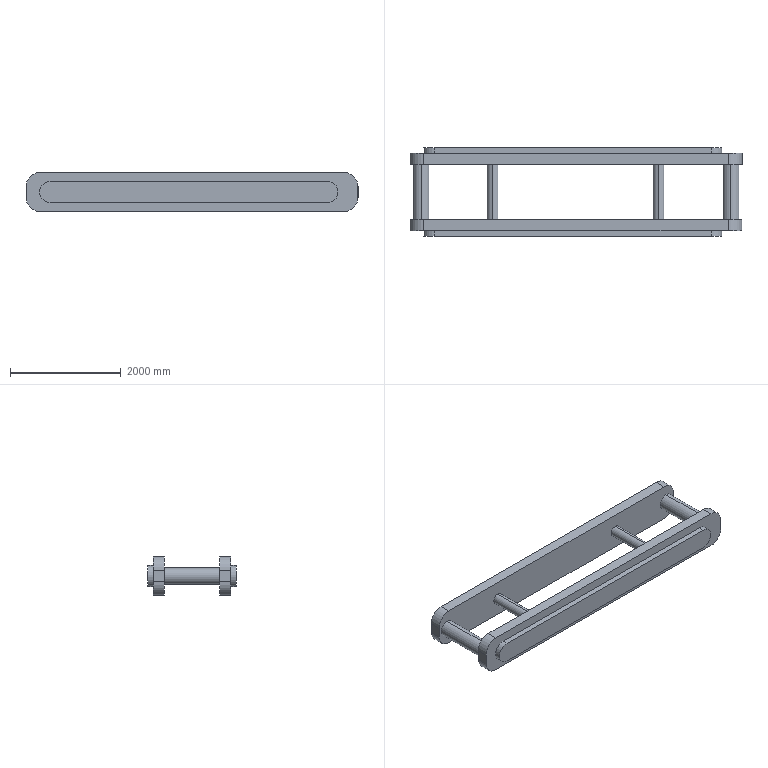Part | SolidWorks | features ICE 3, Extrusion 1, Fillet 1, MirrorPattern 1 | 1 solid | 38 faces | box 6002 x 1600 x 700 mm | volume 2271942121 mm3 | cylinder 20 | plane 18 | commonest cylinder face diameters 500 x8 200 x4 300 x4 384.606 x4
STEP:
#1=CARTESIAN_POINT('',(-2800.,1200.,150.));
#2=VERTEX_POINT('',#1);
#3=CARTESIAN_POINT('',(-2800.,1200.,-150.));
#4=VERTEX_POINT('',#3);
#5=CARTESIAN_POINT('',(-2800.,1200.,0.));
#6=DIRECTION('',(0.,1.,0.));
#7=DIRECTION('',(0.,0.,1.));
#8=AXIS2_PLACEMENT_3D('',#5,#6,#7);
#9=CIRCLE('',#8,150.);
#10=EDGE_CURVE('',#2,#4,#9,.T.);
#11=ORIENTED_EDGE('',*,*,#10,.F.);
#12=CARTESIAN_POINT('',(-2800.,200.,150.));
#13=VERTEX_POINT('',#12);
#14=CARTESIAN_POINT('',(-2800.,1200.,150.));
#15=DIRECTION('',(0.,-1.,0.));
#16=VECTOR('',#15,1000.);
#17=LINE('',#14,#16);
#18=EDGE_CURVE('',#2,#13,#17,.T.);
#19=ORIENTED_EDGE('',*,*,#18,.T.);
#20=CARTESIAN_POINT('',(-2800.,200.,-150.));
#21=VERTEX_POINT('',#20);
#22=CARTESIAN_POINT('',(-2800.,200.,0.));
#23=DIRECTION('',(0.,1.,0.));
#24=DIRECTION('',(0.,0.,1.));
#25=AXIS2_PLACEMENT_3D('',#22,#23,#24);
#26=CIRCLE('',#25,150.);
#27=EDGE_CURVE('',#13,#21,#26,.T.);
#28=ORIENTED_EDGE('',*,*,#27,.T.);
#29=CARTESIAN_POINT('',(-2800.,1200.,-150.));
#30=DIRECTION('',(0.,-1.,0.));
#31=VECTOR('',#30,1000.);
#32=LINE('',#29,#31);
#33=EDGE_CURVE('',#4,#21,#32,.T.);
#34=ORIENTED_EDGE('',*,*,#33,.F.);
#35=EDGE_LOOP('',(#11,#19,#28,#34));
#36=FACE_OUTER_BOUND('',#35,.T.);
#37=CARTESIAN_POINT('',(-2800.,1200.,0.));
#38=DIRECTION('',(0.,-1.,0.));
#39=DIRECTION('',(0.,0.,-1.));
#40=AXIS2_PLACEMENT_3D('',#37,#38,#39);
#41=CYLINDRICAL_SURFACE('',#40,150.);
#42=ADVANCED_FACE('',(#36),#41,.T.);
#43=CARTESIAN_POINT('',(1500.,1200.,100.));
#44=VERTEX_POINT('',#43);
#45=CARTESIAN_POINT('',(1500.,1200.,-100.));
#46=VERTEX_POINT('',#45);
#47=CARTESIAN_POINT('',(1500.,1200.,0.));
#48=DIRECTION('',(0.,1.,0.));
#49=DIRECTION('',(0.,0.,1.));
#50=AXIS2_PLACEMENT_3D('',#47,#48,#49);
#51=CIRCLE('',#50,100.);
#52=EDGE_CURVE('',#44,#46,#51,.T.);
#53=ORIENTED_EDGE('',*,*,#52,.F.);
#54=CARTESIAN_POINT('',(1500.,200.,100.));
#55=VERTEX_POINT('',#54);
#56=CARTESIAN_POINT('',(1500.,1200.,100.));
#57=DIRECTION('',(0.,-1.,0.));
#58=VECTOR('',#57,1000.);
#59=LINE('',#56,#58);
#60=EDGE_CURVE('',#44,#55,#59,.T.);
#61=ORIENTED_EDGE('',*,*,#60,.T.);
#62=CARTESIAN_POINT('',(1500.,200.,-100.));
#63=VERTEX_POINT('',#62);
#64=CARTESIAN_POINT('',(1500.,200.,0.));
#65=DIRECTION('',(0.,1.,0.));
#66=DIRECTION('',(0.,0.,1.));
#67=AXIS2_PLACEMENT_3D('',#64,#65,#66);
#68=CIRCLE('',#67,100.);
#69=EDGE_CURVE('',#55,#63,#68,.T.);
#70=ORIENTED_EDGE('',*,*,#69,.T.);
#71=CARTESIAN_POINT('',(1500.,1200.,-100.));
#72=DIRECTION('',(0.,-1.,0.));
#73=VECTOR('',#72,1000.);
#74=LINE('',#71,#73);
#75=EDGE_CURVE('',#46,#63,#74,.T.);
#76=ORIENTED_EDGE('',*,*,#75,.F.);
#77=EDGE_LOOP('',(#53,#61,#70,#76));
#78=FACE_OUTER_BOUND('',#77,.T.);
#79=CARTESIAN_POINT('',(1500.,1200.,0.));
#80=DIRECTION('',(0.,-1.,0.));
#81=DIRECTION('',(0.,0.,-1.));
#82=AXIS2_PLACEMENT_3D('',#79,#80,#81);
#83=CYLINDRICAL_SURFACE('',#82,100.);
#84=ADVANCED_FACE('',(#78),#83,.T.);
#85=CARTESIAN_POINT('',(-1500.,1200.,100.));
#86=VERTEX_POINT('',#85);
#87=CARTESIAN_POINT('',(-1500.,1200.,-100.));
#88=VERTEX_POINT('',#87);
#89=CARTESIAN_POINT('',(-1500.,1200.,0.));
#90=DIRECTION('',(0.,1.,0.));
#91=DIRECTION('',(0.,0.,1.));
#92=AXIS2_PLACEMENT_3D('',#89,#90,#91);
#93=CIRCLE('',#92,100.);
#94=EDGE_CURVE('',#86,#88,#93,.T.);
#95=ORIENTED_EDGE('',*,*,#94,.F.);
#96=CARTESIAN_POINT('',(-1500.,200.,100.));
#97=VERTEX_POINT('',#96);
#98=CARTESIAN_POINT('',(-1500.,1200.,100.));
#99=DIRECTION('',(0.,-1.,0.));
#100=VECTOR('',#99,1000.);
#101=LINE('',#98,#100);
#102=EDGE_CURVE('',#86,#97,#101,.T.);
#103=ORIENTED_EDGE('',*,*,#102,.T.);
#104=CARTESIAN_POINT('',(-1500.,200.,-100.));
#105=VERTEX_POINT('',#104);
#106=CARTESIAN_POINT('',(-1500.,200.,0.));
#107=DIRECTION('',(0.,1.,0.));
#108=DIRECTION('',(0.,0.,1.));
#109=AXIS2_PLACEMENT_3D('',#106,#107,#108);
#110=CIRCLE('',#109,100.);
#111=EDGE_CURVE('',#97,#105,#110,.T.);
#112=ORIENTED_EDGE('',*,*,#111,.T.);
#113=CARTESIAN_POINT('',(-1500.,1200.,-100.));
#114=DIRECTION('',(0.,-1.,0.));
#115=VECTOR('',#114,1000.);
#116=LINE('',#113,#115);
#117=EDGE_CURVE('',#88,#105,#116,.T.);
#118=ORIENTED_EDGE('',*,*,#117,.F.);
#119=EDGE_LOOP('',(#95,#103,#112,#118));
#120=FACE_OUTER_BOUND('',#119,.T.);
#121=CARTESIAN_POINT('',(-1500.,1200.,0.));
#122=DIRECTION('',(0.,-1.,0.));
#123=DIRECTION('',(0.,0.,-1.));
#124=AXIS2_PLACEMENT_3D('',#121,#122,#123);
#125=CYLINDRICAL_SURFACE('',#124,100.);
#126=ADVANCED_FACE('',(#120),#125,.T.);
#127=CARTESIAN_POINT('',(2800.,1200.,150.));
#128=VERTEX_POINT('',#127);
#129=CARTESIAN_POINT('',(2800.,1200.,-150.));
#130=VERTEX_POINT('',#129);
#131=CARTESIAN_POINT('',(2800.,1200.,0.));
#132=DIRECTION('',(0.,1.,0.));
#133=DIRECTION('',(0.,0.,1.));
#134=AXIS2_PLACEMENT_3D('',#131,#132,#133);
#135=CIRCLE('',#134,150.);
#136=EDGE_CURVE('',#128,#130,#135,.T.);
#137=ORIENTED_EDGE('',*,*,#136,.F.);
#138=CARTESIAN_POINT('',(2800.,200.,150.));
#139=VERTEX_POINT('',#138);
#140=CARTESIAN_POINT('',(2800.,1200.,150.));
#141=DIRECTION('',(0.,-1.,0.));
#142=VECTOR('',#141,1000.);
#143=LINE('',#140,#142);
#144=EDGE_CURVE('',#128,#139,#143,.T.);
#145=ORIENTED_EDGE('',*,*,#144,.T.);
#146=CARTESIAN_POINT('',(2800.,200.,-150.));
#147=VERTEX_POINT('',#146);
#148=CARTESIAN_POINT('',(2800.,200.,0.));
#149=DIRECTION('',(0.,1.,0.));
#150=DIRECTION('',(0.,0.,1.));
#151=AXIS2_PLACEMENT_3D('',#148,#149,#150);
#152=CIRCLE('',#151,150.);
#153=EDGE_CURVE('',#139,#147,#152,.T.);
#154=ORIENTED_EDGE('',*,*,#153,.T.);
#155=CARTESIAN_POINT('',(2800.,1200.,-150.));
#156=DIRECTION('',(0.,-1.,0.));
#157=VECTOR('',#156,1000.);
#158=LINE('',#155,#157);
#159=EDGE_CURVE('',#130,#147,#158,.T.);
#160=ORIENTED_EDGE('',*,*,#159,.F.);
#161=EDGE_LOOP('',(#137,#145,#154,#160));
#162=FACE_OUTER_BOUND('',#161,.T.);
#163=CARTESIAN_POINT('',(2800.,1200.,0.));
#164=DIRECTION('',(0.,-1.,0.));
#165=DIRECTION('',(0.,0.,-1.));
#166=AXIS2_PLACEMENT_3D('',#163,#164,#165);
#167=CYLINDRICAL_SURFACE('',#166,150.);
#168=ADVANCED_FACE('',(#162),#167,.T.);
#169=CARTESIAN_POINT('',(2750.,0.,-350.));
#170=VERTEX_POINT('',#169);
#171=CARTESIAN_POINT('',(-2750.,0.,-350.));
#172=VERTEX_POINT('',#171);
#173=CARTESIAN_POINT('',(-3000.,0.,-350.));
#174=DIRECTION('',(-1.,0.,0.));
#175=VECTOR('',#174,1000.);
#176=LINE('',#173,#175);
#177=EDGE_CURVE('',#170,#172,#176,.T.);
#178=ORIENTED_EDGE('',*,*,#177,.F.);
#179=CARTESIAN_POINT('',(3000.,0.,-100.));
#180=VERTEX_POINT('',#179);
#181=CARTESIAN_POINT('',(2750.,0.,-100.));
#182=DIRECTION('',(0.,-1.,0.));
#183=DIRECTION('',(0.,0.,1.));
#184=AXIS2_PLACEMENT_3D('',#181,#182,#183);
#185=CIRCLE('',#184,250.);
#186=EDGE_CURVE('',#170,#180,#185,.T.);
#187=ORIENTED_EDGE('',*,*,#186,.T.);
#188=CARTESIAN_POINT('',(3000.,0.,100.));
#189=VERTEX_POINT('',#188);
#190=CARTESIAN_POINT('',(3000.,0.,-350.));
#191=DIRECTION('',(0.,0.,-1.));
#192=VECTOR('',#191,1000.);
#193=LINE('',#190,#192);
#194=EDGE_CURVE('',#189,#180,#193,.T.);
#195=ORIENTED_EDGE('',*,*,#194,.F.);
#196=CARTESIAN_POINT('',(2750.,0.,350.));
#197=VERTEX_POINT('',#196);
#198=CARTESIAN_POINT('',(2750.,0.,100.));
#199=DIRECTION('',(0.,-1.,0.));
#200=DIRECTION('',(0.,0.,1.));
#201=AXIS2_PLACEMENT_3D('',#198,#199,#200);
#202=CIRCLE('',#201,250.);
#203=EDGE_CURVE('',#189,#197,#202,.T.);
#204=ORIENTED_EDGE('',*,*,#203,.T.);
#205=CARTESIAN_POINT('',(-2750.,0.,350.));
#206=VERTEX_POINT('',#205);
#207=CARTESIAN_POINT('',(-3000.,0.,350.));
#208=DIRECTION('',(1.,0.,0.));
#209=VECTOR('',#208,1000.);
#210=LINE('',#207,#209);
#211=EDGE_CURVE('',#206,#197,#210,.T.);
#212=ORIENTED_EDGE('',*,*,#211,.F.);
#213=CARTESIAN_POINT('',(-3000.,0.,100.));
#214=VERTEX_POINT('',#213);
#215=CARTESIAN_POINT('',(-2750.,0.,100.));
#216=DIRECTION('',(0.,-1.,0.));
#217=DIRECTION('',(0.,0.,1.));
#218=AXIS2_PLACEMENT_3D('',#215,#216,#217);
#219=CIRCLE('',#218,250.);
#220=EDGE_CURVE('',#206,#214,#219,.T.);
#221=ORIENTED_EDGE('',*,*,#220,.T.);
#222=CARTESIAN_POINT('',(-3000.,0.,-100.));
#223=VERTEX_POINT('',#222);
#224=CARTESIAN_POINT('',(-3000.,0.,-350.));
#225=DIRECTION('',(0.,0.,1.));
#226=VECTOR('',#225,1000.);
#227=LINE('',#224,#226);
#228=EDGE_CURVE('',#223,#214,#227,.T.);
#229=ORIENTED_EDGE('',*,*,#228,.F.);
#230=CARTESIAN_POINT('',(-2750.,0.,-100.));
#231=DIRECTION('',(0.,-1.,0.));
#232=DIRECTION('',(0.,0.,1.));
#233=AXIS2_PLACEMENT_3D('',#230,#231,#232);
#234=CIRCLE('',#233,250.);
#235=EDGE_CURVE('',#223,#172,#234,.T.);
#236=ORIENTED_EDGE('',*,*,#235,.T.);
#237=EDGE_LOOP('',(#178,#187,#195,#204,#212,#221,#229,#236));
#238=FACE_OUTER_BOUND('',#237,.T.);
#239=CARTESIAN_POINT('',(-2564.073,0.,192.303));
#240=VERTEX_POINT('',#239);
#241=CARTESIAN_POINT('',(-2564.073,0.,-192.303));
#242=VERTEX_POINT('',#241);
#243=CARTESIAN_POINT('',(-2564.073,0.,0.));
#244=DIRECTION('',(0.,-1.,0.));
#245=DIRECTION('',(0.,0.,-1.));
#246=AXIS2_PLACEMENT_3D('',#243,#244,#245);
#247=CIRCLE('',#246,192.303);
#248=EDGE_CURVE('',#240,#242,#247,.T.);
#249=ORIENTED_EDGE('',*,*,#248,.F.);
#250=CARTESIAN_POINT('',(2449.537,0.,192.303));
#251=VERTEX_POINT('',#250);
#252=CARTESIAN_POINT('',(-2564.073,0.,192.303));
#253=DIRECTION('',(-1.,0.,0.));
#254=VECTOR('',#253,1000.);
#255=LINE('',#252,#254);
#256=EDGE_CURVE('',#251,#240,#255,.T.);
#257=ORIENTED_EDGE('',*,*,#256,.F.);
#258=CARTESIAN_POINT('',(2449.537,0.,-192.303));
#259=VERTEX_POINT('',#258);
#260=CARTESIAN_POINT('',(2449.537,0.,0.));
#261=DIRECTION('',(0.,-1.,0.));
#262=DIRECTION('',(0.,0.,-1.));
#263=AXIS2_PLACEMENT_3D('',#260,#261,#262);
#264=CIRCLE('',#263,192.303);
#265=EDGE_CURVE('',#259,#251,#264,.T.);
#266=ORIENTED_EDGE('',*,*,#265,.F.);
#267=CARTESIAN_POINT('',(-2564.073,0.,-192.303));
#268=DIRECTION('',(1.,0.,0.));
#269=VECTOR('',#268,1000.);
#270=LINE('',#267,#269);
#271=EDGE_CURVE('',#242,#259,#270,.T.);
#272=ORIENTED_EDGE('',*,*,#271,.F.);
#273=EDGE_LOOP('',(#249,#257,#266,#272));
#274=FACE_BOUND('',#273,.T.);
#275=CARTESIAN_POINT('',(0.,0.,0.));
#276=DIRECTION('',(0.,1.,0.));
#277=DIRECTION('',(0.,0.,1.));
#278=AXIS2_PLACEMENT_3D('',#275,#276,#277);
#279=PLANE('',#278);
#280=ADVANCED_FACE('',(#238,#274),#279,.F.);
#281=ORIENTED_EDGE('',*,*,#194,.T.);
#282=CARTESIAN_POINT('',(3000.,200.,-100.));
#283=VERTEX_POINT('',#282);
#284=CARTESIAN_POINT('',(3000.,200.,-100.));
#285=DIRECTION('',(0.,1.,0.));
#286=VECTOR('',#285,1000.);
#287=LINE('',#284,#286);
#288=EDGE_CURVE('',#180,#283,#287,.T.);
#289=ORIENTED_EDGE('',*,*,#288,.T.);
#290=CARTESIAN_POINT('',(3000.,200.,100.));
#291=VERTEX_POINT('',#290);
#292=CARTESIAN_POINT('',(3000.,200.,-350.));
#293=DIRECTION('',(0.,0.,-1.));
#294=VECTOR('',#293,1000.);
#295=LINE('',#292,#294);
#296=EDGE_CURVE('',#291,#283,#295,.T.);
#297=ORIENTED_EDGE('',*,*,#296,.F.);
#298=CARTESIAN_POINT('',(3000.,200.,100.));
#299=DIRECTION('',(0.,-1.,0.));
#300=VECTOR('',#299,1000.);
#301=LINE('',#298,#300);
#302=EDGE_CURVE('',#291,#189,#301,.T.);
#303=ORIENTED_EDGE('',*,*,#302,.T.);
#304=EDGE_LOOP('',(#281,#289,#297,#303));
#305=FACE_OUTER_BOUND('',#304,.T.);
#306=CARTESIAN_POINT('',(3000.,200.,-350.));
#307=DIRECTION('',(-1.,0.,0.));
#308=DIRECTION('',(0.,0.,1.));
#309=AXIS2_PLACEMENT_3D('',#306,#307,#308);
#310=PLANE('',#309);
#311=ADVANCED_FACE('',(#305),#310,.F.);
#312=CARTESIAN_POINT('',(2750.,200.,-350.));
#313=VERTEX_POINT('',#312);
#314=CARTESIAN_POINT('',(-2750.,200.,-350.));
#315=VERTEX_POINT('',#314);
#316=CARTESIAN_POINT('',(-3000.,200.,-350.));
#317=DIRECTION('',(-1.,0.,0.));
#318=VECTOR('',#317,1000.);
#319=LINE('',#316,#318);
#320=EDGE_CURVE('',#313,#315,#319,.T.);
#321=ORIENTED_EDGE('',*,*,#320,.F.);
#322=CARTESIAN_POINT('',(2750.,200.,-350.));
#323=DIRECTION('',(0.,-1.,0.));
#324=VECTOR('',#323,1000.);
#325=LINE('',#322,#324);
#326=EDGE_CURVE('',#313,#170,#325,.T.);
#327=ORIENTED_EDGE('',*,*,#326,.T.);
#328=ORIENTED_EDGE('',*,*,#177,.T.);
#329=CARTESIAN_POINT('',(-2750.,200.,-350.));
#330=DIRECTION('',(0.,1.,0.));
#331=VECTOR('',#330,1000.);
#332=LINE('',#329,#331);
#333=EDGE_CURVE('',#172,#315,#332,.T.);
#334=ORIENTED_EDGE('',*,*,#333,.T.);
#335=EDGE_LOOP('',(#321,#327,#328,#334));
#336=FACE_OUTER_BOUND('',#335,.T.);
#337=CARTESIAN_POINT('',(-3000.,200.,-350.));
#338=DIRECTION('',(0.,0.,1.));
#339=DIRECTION('',(1.,0.,0.));
#340=AXIS2_PLACEMENT_3D('',#337,#338,#339);
#341=PLANE('',#340);
#342=ADVANCED_FACE('',(#336),#341,.F.);
#343=CARTESIAN_POINT('',(-3000.,200.,-100.));
#344=VERTEX_POINT('',#343);
#345=CARTESIAN_POINT('',(-3000.,200.,100.));
#346=VERTEX_POINT('',#345);
#347=CARTESIAN_POINT('',(-3000.,200.,-350.));
#348=DIRECTION('',(0.,0.,1.));
#349=VECTOR('',#348,1000.);
#350=LINE('',#347,#349);
#351=EDGE_CURVE('',#344,#346,#350,.T.);
#352=ORIENTED_EDGE('',*,*,#351,.F.);
#353=CARTESIAN_POINT('',(-3000.,200.,-100.));
#354=DIRECTION('',(0.,-1.,0.));
#355=VECTOR('',#354,1000.);
#356=LINE('',#353,#355);
#357=EDGE_CURVE('',#344,#223,#356,.T.);
#358=ORIENTED_EDGE('',*,*,#357,.T.);
#359=ORIENTED_EDGE('',*,*,#228,.T.);
#360=CARTESIAN_POINT('',(-3000.,200.,100.));
#361=DIRECTION('',(0.,1.,0.));
#362=VECTOR('',#361,1000.);
#363=LINE('',#360,#362);
#364=EDGE_CURVE('',#214,#346,#363,.T.);
#365=ORIENTED_EDGE('',*,*,#364,.T.);
#366=EDGE_LOOP('',(#352,#358,#359,#365));
#367=FACE_OUTER_BOUND('',#366,.T.);
#368=CARTESIAN_POINT('',(-3000.,200.,-350.));
#369=DIRECTION('',(1.,0.,0.));
#370=DIRECTION('',(0.,0.,-1.));
#371=AXIS2_PLACEMENT_3D('',#368,#369,#370);
#372=PLANE('',#371);
#373=ADVANCED_FACE('',(#367),#372,.F.);
#374=ORIENTED_EDGE('',*,*,#211,.T.);
#375=CARTESIAN_POINT('',(2750.,200.,350.));
#376=VERTEX_POINT('',#375);
#377=CARTESIAN_POINT('',(2750.,200.,350.));
#378=DIRECTION('',(0.,1.,0.));
#379=VECTOR('',#378,1000.);
#380=LINE('',#377,#379);
#381=EDGE_CURVE('',#197,#376,#380,.T.);
#382=ORIENTED_EDGE('',*,*,#381,.T.);
#383=CARTESIAN_POINT('',(-2750.,200.,350.));
#384=VERTEX_POINT('',#383);
#385=CARTESIAN_POINT('',(-3000.,200.,350.));
#386=DIRECTION('',(1.,0.,0.));
#387=VECTOR('',#386,1000.);
#388=LINE('',#385,#387);
#389=EDGE_CURVE('',#384,#376,#388,.T.);
#390=ORIENTED_EDGE('',*,*,#389,.F.);
#391=CARTESIAN_POINT('',(-2750.,200.,350.));
#392=DIRECTION('',(0.,-1.,0.));
#393=VECTOR('',#392,1000.);
#394=LINE('',#391,#393);
#395=EDGE_CURVE('',#384,#206,#394,.T.);
#396=ORIENTED_EDGE('',*,*,#395,.T.);
#397=EDGE_LOOP('',(#374,#382,#390,#396));
#398=FACE_OUTER_BOUND('',#397,.T.);
#399=CARTESIAN_POINT('',(-3000.,200.,350.));
#400=DIRECTION('',(0.,0.,-1.));
#401=DIRECTION('',(-1.,0.,0.));
#402=AXIS2_PLACEMENT_3D('',#399,#400,#401);
#403=PLANE('',#402);
#404=ADVANCED_FACE('',(#398),#403,.F.);
#405=CARTESIAN_POINT('',(-2800.,200.,0.));
#406=DIRECTION('',(0.,1.,0.));
#407=DIRECTION('',(0.,0.,1.));
#408=AXIS2_PLACEMENT_3D('',#405,#406,#407);
#409=CIRCLE('',#408,150.);
#410=EDGE_CURVE('',#21,#13,#409,.T.);
#411=ORIENTED_EDGE('',*,*,#410,.F.);
#412=ORIENTED_EDGE('',*,*,#27,.F.);
#413=EDGE_LOOP('',(#411,#412));
#414=FACE_BOUND('',#413,.T.);
#415=CARTESIAN_POINT('',(1500.,200.,0.));
#416=DIRECTION('',(0.,1.,0.));
#417=DIRECTION('',(0.,0.,1.));
#418=AXIS2_PLACEMENT_3D('',#415,#416,#417);
#419=CIRCLE('',#418,100.);
#420=EDGE_CURVE('',#63,#55,#419,.T.);
#421=ORIENTED_EDGE('',*,*,#420,.F.);
#422=ORIENTED_EDGE('',*,*,#69,.F.);
#423=EDGE_LOOP('',(#421,#422));
#424=FACE_BOUND('',#423,.T.);
#425=CARTESIAN_POINT('',(-1500.,200.,0.));
#426=DIRECTION('',(0.,1.,0.));
#427=DIRECTION('',(0.,0.,1.));
#428=AXIS2_PLACEMENT_3D('',#425,#426,#427);
#429=CIRCLE('',#428,100.);
#430=EDGE_CURVE('',#105,#97,#429,.T.);
#431=ORIENTED_EDGE('',*,*,#430,.F.);
#432=ORIENTED_EDGE('',*,*,#111,.F.);
#433=EDGE_LOOP('',(#431,#432));
#434=FACE_BOUND('',#433,.T.);
#435=CARTESIAN_POINT('',(2800.,200.,0.));
#436=DIRECTION('',(0.,1.,0.));
#437=DIRECTION('',(0.,0.,1.));
#438=AXIS2_PLACEMENT_3D('',#435,#436,#437);
#439=CIRCLE('',#438,150.);
#440=EDGE_CURVE('',#147,#139,#439,.T.);
#441=ORIENTED_EDGE('',*,*,#440,.F.);
#442=ORIENTED_EDGE('',*,*,#153,.F.);
#443=EDGE_LOOP('',(#441,#442));
#444=FACE_BOUND('',#443,.T.);
#445=ORIENTED_EDGE('',*,*,#296,.T.);
#446=CARTESIAN_POINT('',(2750.,200.,-100.));
#447=DIRECTION('',(0.,1.,0.));
#448=DIRECTION('',(0.,0.,1.));
#449=AXIS2_PLACEMENT_3D('',#446,#447,#448);
#450=CIRCLE('',#449,250.);
#451=EDGE_CURVE('',#283,#313,#450,.T.);
#452=ORIENTED_EDGE('',*,*,#451,.T.);
#453=ORIENTED_EDGE('',*,*,#320,.T.);
#454=CARTESIAN_POINT('',(-2750.,200.,-100.));
#455=DIRECTION('',(0.,1.,0.));
#456=DIRECTION('',(0.,0.,1.));
#457=AXIS2_PLACEMENT_3D('',#454,#455,#456);
#458=CIRCLE('',#457,250.);
#459=EDGE_CURVE('',#315,#344,#458,.T.);
#460=ORIENTED_EDGE('',*,*,#459,.T.);
#461=ORIENTED_EDGE('',*,*,#351,.T.);
#462=CARTESIAN_POINT('',(-2750.,200.,100.));
#463=DIRECTION('',(0.,1.,0.));
#464=DIRECTION('',(0.,0.,1.));
#465=AXIS2_PLACEMENT_3D('',#462,#463,#464);
#466=CIRCLE('',#465,250.);
#467=EDGE_CURVE('',#346,#384,#466,.T.);
#468=ORIENTED_EDGE('',*,*,#467,.T.);
#469=ORIENTED_EDGE('',*,*,#389,.T.);
#470=CARTESIAN_POINT('',(2750.,200.,100.));
#471=DIRECTION('',(0.,1.,0.));
#472=DIRECTION('',(0.,0.,1.));
#473=AXIS2_PLACEMENT_3D('',#470,#471,#472);
#474=CIRCLE('',#473,250.);
#475=EDGE_CURVE('',#376,#291,#474,.T.);
#476=ORIENTED_EDGE('',*,*,#475,.T.);
#477=EDGE_LOOP('',(#445,#452,#453,#460,#461,#468,#469,#476));
#478=FACE_OUTER_BOUND('',#477,.T.);
#479=CARTESIAN_POINT('',(0.,200.,0.));
#480=DIRECTION('',(0.,1.,0.));
#481=DIRECTION('',(0.,0.,1.));
#482=AXIS2_PLACEMENT_3D('',#479,#480,#481);
#483=PLANE('',#482);
#484=ADVANCED_FACE('',(#414,#424,#434,#444,#478),#483,.T.);
#485=ORIENTED_EDGE('',*,*,#144,.F.);
#486=CARTESIAN_POINT('',(2800.,1200.,0.));
#487=DIRECTION('',(0.,1.,0.));
#488=DIRECTION('',(0.,0.,1.));
#489=AXIS2_PLACEMENT_3D('',#486,#487,#488);
#490=CIRCLE('',#489,150.);
#491=EDGE_CURVE('',#130,#128,#490,.T.);
#492=ORIENTED_EDGE('',*,*,#491,.F.);
#493=ORIENTED_EDGE('',*,*,#159,.T.);
#494=ORIENTED_EDGE('',*,*,#440,.T.);
#495=EDGE_LOOP('',(#485,#492,#493,#494));
#496=FACE_OUTER_BOUND('',#495,.T.);
#497=CARTESIAN_POINT('',(2800.,1200.,0.));
#498=DIRECTION('',(0.,-1.,0.));
#499=DIRECTION('',(0.,0.,-1.));
#500=AXIS2_PLACEMENT_3D('',#497,#498,#499);
#501=CYLINDRICAL_SURFACE('',#500,150.);
#502=ADVANCED_FACE('',(#496),#501,.T.);
#503=ORIENTED_EDGE('',*,*,#102,.F.);
#504=CARTESIAN_POINT('',(-1500.,1200.,0.));
#505=DIRECTION('',(0.,1.,0.));
#506=DIRECTION('',(0.,0.,1.));
#507=AXIS2_PLACEMENT_3D('',#504,#505,#506);
#508=CIRCLE('',#507,100.);
#509=EDGE_CURVE('',#88,#86,#508,.T.);
#510=ORIENTED_EDGE('',*,*,#509,.F.);
#511=ORIENTED_EDGE('',*,*,#117,.T.);
#512=ORIENTED_EDGE('',*,*,#430,.T.);
#513=EDGE_LOOP('',(#503,#510,#511,#512));
#514=FACE_OUTER_BOUND('',#513,.T.);
#515=CARTESIAN_POINT('',(-1500.,1200.,0.));
#516=DIRECTION('',(0.,-1.,0.));
#517=DIRECTION('',(0.,0.,-1.));
#518=AXIS2_PLACEMENT_3D('',#515,#516,#517);
#519=CYLINDRICAL_SURFACE('',#518,100.);
#520=ADVANCED_FACE('',(#514),#519,.T.);
#521=ORIENTED_EDGE('',*,*,#60,.F.);
#522=CARTESIAN_POINT('',(1500.,1200.,0.));
#523=DIRECTION('',(0.,1.,0.));
#524=DIRECTION('',(0.,0.,1.));
#525=AXIS2_PLACEMENT_3D('',#522,#523,#524);
#526=CIRCLE('',#525,100.);
#527=EDGE_CURVE('',#46,#44,#526,.T.);
#528=ORIENTED_EDGE('',*,*,#527,.F.);
#529=ORIENTED_EDGE('',*,*,#75,.T.);
#530=ORIENTED_EDGE('',*,*,#420,.T.);
#531=EDGE_LOOP('',(#521,#528,#529,#530));
#532=FACE_OUTER_BOUND('',#531,.T.);
#533=CARTESIAN_POINT('',(1500.,1200.,0.));
#534=DIRECTION('',(0.,-1.,0.));
#535=DIRECTION('',(0.,0.,-1.));
#536=AXIS2_PLACEMENT_3D('',#533,#534,#535);
#537=CYLINDRICAL_SURFACE('',#536,100.);
#538=ADVANCED_FACE('',(#532),#537,.T.);
#539=ORIENTED_EDGE('',*,*,#18,.F.);
#540=CARTESIAN_POINT('',(-2800.,1200.,0.));
#541=DIRECTION('',(0.,1.,0.));
#542=DIRECTION('',(0.,0.,1.));
#543=AXIS2_PLACEMENT_3D('',#540,#541,#542);
#544=CIRCLE('',#543,150.);
#545=EDGE_CURVE('',#4,#2,#544,.T.);
#546=ORIENTED_EDGE('',*,*,#545,.F.);
#547=ORIENTED_EDGE('',*,*,#33,.T.);
#548=ORIENTED_EDGE('',*,*,#410,.T.);
#549=EDGE_LOOP('',(#539,#546,#547,#548));
#550=FACE_OUTER_BOUND('',#549,.T.);
#551=CARTESIAN_POINT('',(-2800.,1200.,0.));
#552=DIRECTION('',(0.,-1.,0.));
#553=DIRECTION('',(0.,0.,-1.));
#554=AXIS2_PLACEMENT_3D('',#551,#552,#553);
#555=CYLINDRICAL_SURFACE('',#554,150.);
#556=ADVANCED_FACE('',(#550),#555,.T.);
#557=CARTESIAN_POINT('',(2752.219,1400.,-350.));
#558=VERTEX_POINT('',#557);
#559=CARTESIAN_POINT('',(-2750.,1400.,-350.));
#560=VERTEX_POINT('',#559);
#561=CARTESIAN_POINT('',(-3000.,1400.,-350.));
#562=DIRECTION('',(-1.,0.,0.));
#563=VECTOR('',#562,1000.);
#564=LINE('',#561,#563);
#565=EDGE_CURVE('',#558,#560,#564,.T.);
#566=ORIENTED_EDGE('',*,*,#565,.F.);
#567=CARTESIAN_POINT('',(2752.219,1200.,-350.));
#568=VERTEX_POINT('',#567);
#569=CARTESIAN_POINT('',(2752.219,1400.,-350.));
#570=DIRECTION('',(0.,-1.,0.));
#571=VECTOR('',#570,1000.);
#572=LINE('',#569,#571);
#573=EDGE_CURVE('',#558,#568,#572,.T.);
#574=ORIENTED_EDGE('',*,*,#573,.T.);
#575=CARTESIAN_POINT('',(-2750.,1200.,-350.));
#576=VERTEX_POINT('',#575);
#577=CARTESIAN_POINT('',(-3000.,1200.,-350.));
#578=DIRECTION('',(-1.,0.,0.));
#579=VECTOR('',#578,1000.);
#580=LINE('',#577,#579);
#581=EDGE_CURVE('',#568,#576,#580,.T.);
#582=ORIENTED_EDGE('',*,*,#581,.T.);
#583=CARTESIAN_POINT('',(-2750.,1400.,-350.));
#584=DIRECTION('',(0.,1.,0.));
#585=VECTOR('',#584,1000.);
#586=LINE('',#583,#585);
#587=EDGE_CURVE('',#576,#560,#586,.T.);
#588=ORIENTED_EDGE('',*,*,#587,.T.);
#589=EDGE_LOOP('',(#566,#574,#582,#588));
#590=FACE_OUTER_BOUND('',#589,.T.);
#591=CARTESIAN_POINT('',(-3000.,1400.,-350.));
#592=DIRECTION('',(0.,0.,1.));
#593=DIRECTION('',(1.,0.,0.));
#594=AXIS2_PLACEMENT_3D('',#591,#592,#593);
#595=PLANE('',#594);
#596=ADVANCED_FACE('',(#590),#595,.F.);
#597=CARTESIAN_POINT('',(-3000.,1400.,-100.));
#598=VERTEX_POINT('',#597);
#599=CARTESIAN_POINT('',(-3000.,1400.,100.));
#600=VERTEX_POINT('',#599);
#601=CARTESIAN_POINT('',(-3000.,1400.,-350.));
#602=DIRECTION('',(0.,0.,1.));
#603=VECTOR('',#602,1000.);
#604=LINE('',#601,#603);
#605=EDGE_CURVE('',#598,#600,#604,.T.);
#606=ORIENTED_EDGE('',*,*,#605,.F.);
#607=CARTESIAN_POINT('',(-3000.,1200.,-100.));
#608=VERTEX_POINT('',#607);
#609=CARTESIAN_POINT('',(-3000.,1400.,-100.));
#610=DIRECTION('',(0.,-1.,0.));
#611=VECTOR('',#610,1000.);
#612=LINE('',#609,#611);
#613=EDGE_CURVE('',#598,#608,#612,.T.);
#614=ORIENTED_EDGE('',*,*,#613,.T.);
#615=CARTESIAN_POINT('',(-3000.,1200.,100.));
#616=VERTEX_POINT('',#615);
#617=CARTESIAN_POINT('',(-3000.,1200.,-350.));
#618=DIRECTION('',(0.,0.,1.));
#619=VECTOR('',#618,1000.);
#620=LINE('',#617,#619);
#621=EDGE_CURVE('',#608,#616,#620,.T.);
#622=ORIENTED_EDGE('',*,*,#621,.T.);
#623=CARTESIAN_POINT('',(-3000.,1400.,100.));
#624=DIRECTION('',(0.,1.,0.));
#625=VECTOR('',#624,1000.);
#626=LINE('',#623,#625);
#627=EDGE_CURVE('',#616,#600,#626,.T.);
#628=ORIENTED_EDGE('',*,*,#627,.T.);
#629=EDGE_LOOP('',(#606,#614,#622,#628));
#630=FACE_OUTER_BOUND('',#629,.T.);
#631=CARTESIAN_POINT('',(-3000.,1400.,-350.));
#632=DIRECTION('',(1.,0.,0.));
#633=DIRECTION('',(0.,0.,-1.));
#634=AXIS2_PLACEMENT_3D('',#631,#632,#633);
#635=PLANE('',#634);
#636=ADVANCED_FACE('',(#630),#635,.F.);
#637=CARTESIAN_POINT('',(-2750.,1200.,350.));
#638=VERTEX_POINT('',#637);
#639=CARTESIAN_POINT('',(2752.219,1200.,350.));
#640=VERTEX_POINT('',#639);
#641=CARTESIAN_POINT('',(-3000.,1200.,350.));
#642=DIRECTION('',(1.,0.,0.));
#643=VECTOR('',#642,1000.);
#644=LINE('',#641,#643);
#645=EDGE_CURVE('',#638,#640,#644,.T.);
#646=ORIENTED_EDGE('',*,*,#645,.T.);
#647=CARTESIAN_POINT('',(2752.219,1400.,350.));
#648=VERTEX_POINT('',#647);
#649=CARTESIAN_POINT('',(2752.219,1400.,350.));
#650=DIRECTION('',(0.,1.,0.));
#651=VECTOR('',#650,1000.);
#652=LINE('',#649,#651);
#653=EDGE_CURVE('',#640,#648,#652,.T.);
#654=ORIENTED_EDGE('',*,*,#653,.T.);
#655=CARTESIAN_POINT('',(-2750.,1400.,350.));
#656=VERTEX_POINT('',#655);
#657=CARTESIAN_POINT('',(-3000.,1400.,350.));
#658=DIRECTION('',(1.,0.,0.));
#659=VECTOR('',#658,1000.);
#660=LINE('',#657,#659);
#661=EDGE_CURVE('',#656,#648,#660,.T.);
#662=ORIENTED_EDGE('',*,*,#661,.F.);
#663=CARTESIAN_POINT('',(-2750.,1400.,350.));
#664=DIRECTION('',(0.,-1.,0.));
#665=VECTOR('',#664,1000.);
#666=LINE('',#663,#665);
#667=EDGE_CURVE('',#656,#638,#666,.T.);
#668=ORIENTED_EDGE('',*,*,#667,.T.);
#669=EDGE_LOOP('',(#646,#654,#662,#668));
#670=FACE_OUTER_BOUND('',#669,.T.);
#671=CARTESIAN_POINT('',(-3000.,1400.,350.));
#672=DIRECTION('',(0.,0.,-1.));
#673=DIRECTION('',(-1.,0.,0.));
#674=AXIS2_PLACEMENT_3D('',#671,#672,#673);
#675=PLANE('',#674);
#676=ADVANCED_FACE('',(#670),#675,.F.);
#677=CARTESIAN_POINT('',(3002.219,1200.,100.));
#678=VERTEX_POINT('',#677);
#679=CARTESIAN_POINT('',(3002.219,1200.,-100.));
#680=VERTEX_POINT('',#679);
#681=CARTESIAN_POINT('',(3002.219,1200.,-350.));
#682=DIRECTION('',(0.,0.,-1.));
#683=VECTOR('',#682,1000.);
#684=LINE('',#681,#683);
#685=EDGE_CURVE('',#678,#680,#684,.T.);
#686=ORIENTED_EDGE('',*,*,#685,.T.);
#687=CARTESIAN_POINT('',(3002.219,1400.,-100.));
#688=VERTEX_POINT('',#687);
#689=CARTESIAN_POINT('',(3002.219,1400.,-100.));
#690=DIRECTION('',(0.,1.,0.));
#691=VECTOR('',#690,1000.);
#692=LINE('',#689,#691);
#693=EDGE_CURVE('',#680,#688,#692,.T.);
#694=ORIENTED_EDGE('',*,*,#693,.T.);
#695=CARTESIAN_POINT('',(3002.219,1400.,100.));
#696=VERTEX_POINT('',#695);
#697=CARTESIAN_POINT('',(3002.219,1400.,-350.));
#698=DIRECTION('',(0.,0.,-1.));
#699=VECTOR('',#698,1000.);
#700=LINE('',#697,#699);
#701=EDGE_CURVE('',#696,#688,#700,.T.);
#702=ORIENTED_EDGE('',*,*,#701,.F.);
#703=CARTESIAN_POINT('',(3002.219,1400.,100.));
#704=DIRECTION('',(0.,-1.,0.));
#705=VECTOR('',#704,1000.);
#706=LINE('',#703,#705);
#707=EDGE_CURVE('',#696,#678,#706,.T.);
#708=ORIENTED_EDGE('',*,*,#707,.T.);
#709=EDGE_LOOP('',(#686,#694,#702,#708));
#710=FACE_OUTER_BOUND('',#709,.T.);
#711=CARTESIAN_POINT('',(3002.219,1400.,-350.));
#712=DIRECTION('',(-1.,0.,0.));
#713=DIRECTION('',(0.,0.,1.));
#714=AXIS2_PLACEMENT_3D('',#711,#712,#713);
#715=PLANE('',#714);
#716=ADVANCED_FACE('',(#710),#715,.F.);
#717=CARTESIAN_POINT('',(2449.537,1400.,192.303));
#718=VERTEX_POINT('',#717);
#719=CARTESIAN_POINT('',(-2564.073,1400.,192.303));
#720=VERTEX_POINT('',#719);
#721=CARTESIAN_POINT('',(-2564.073,1400.,192.303));
#722=DIRECTION('',(-1.,0.,0.));
#723=VECTOR('',#722,1000.);
#724=LINE('',#721,#723);
#725=EDGE_CURVE('',#718,#720,#724,.T.);
#726=ORIENTED_EDGE('',*,*,#725,.T.);
#727=CARTESIAN_POINT('',(-2564.073,1400.,-192.303));
#728=VERTEX_POINT('',#727);
#729=CARTESIAN_POINT('',(-2564.073,1400.,0.));
#730=DIRECTION('',(0.,-1.,0.));
#731=DIRECTION('',(0.,0.,-1.));
#732=AXIS2_PLACEMENT_3D('',#729,#730,#731);
#733=CIRCLE('',#732,192.303);
#734=EDGE_CURVE('',#720,#728,#733,.T.);
#735=ORIENTED_EDGE('',*,*,#734,.T.);
#736=CARTESIAN_POINT('',(2449.537,1400.,-192.303));
#737=VERTEX_POINT('',#736);
#738=CARTESIAN_POINT('',(-2564.073,1400.,-192.303));
#739=DIRECTION('',(1.,0.,0.));
#740=VECTOR('',#739,1000.);
#741=LINE('',#738,#740);
#742=EDGE_CURVE('',#728,#737,#741,.T.);
#743=ORIENTED_EDGE('',*,*,#742,.T.);
#744=CARTESIAN_POINT('',(2449.537,1400.,0.));
#745=DIRECTION('',(0.,-1.,0.));
#746=DIRECTION('',(0.,0.,-1.));
#747=AXIS2_PLACEMENT_3D('',#744,#745,#746);
#748=CIRCLE('',#747,192.303);
#749=EDGE_CURVE('',#737,#718,#748,.T.);
#750=ORIENTED_EDGE('',*,*,#749,.T.);
#751=EDGE_LOOP('',(#726,#735,#743,#750));
#752=FACE_BOUND('',#751,.T.);
#753=ORIENTED_EDGE('',*,*,#701,.T.);
#754=CARTESIAN_POINT('',(2752.219,1400.,-100.));
#755=DIRECTION('',(0.,1.,0.));
#756=DIRECTION('',(0.,0.,-1.));
#757=AXIS2_PLACEMENT_3D('',#754,#755,#756);
#758=CIRCLE('',#757,250.);
#759=EDGE_CURVE('',#688,#558,#758,.T.);
#760=ORIENTED_EDGE('',*,*,#759,.T.);
#761=ORIENTED_EDGE('',*,*,#565,.T.);
#762=CARTESIAN_POINT('',(-2750.,1400.,-100.));
#763=DIRECTION('',(0.,1.,0.));
#764=DIRECTION('',(0.,0.,-1.));
#765=AXIS2_PLACEMENT_3D('',#762,#763,#764);
#766=CIRCLE('',#765,250.);
#767=EDGE_CURVE('',#560,#598,#766,.T.);
#768=ORIENTED_EDGE('',*,*,#767,.T.);
#769=ORIENTED_EDGE('',*,*,#605,.T.);
#770=CARTESIAN_POINT('',(-2750.,1400.,100.));
#771=DIRECTION('',(0.,1.,0.));
#772=DIRECTION('',(0.,0.,-1.));
#773=AXIS2_PLACEMENT_3D('',#770,#771,#772);
#774=CIRCLE('',#773,250.);
#775=EDGE_CURVE('',#600,#656,#774,.T.);
#776=ORIENTED_EDGE('',*,*,#775,.T.);
#777=ORIENTED_EDGE('',*,*,#661,.T.);
#778=CARTESIAN_POINT('',(2752.219,1400.,100.));
#779=DIRECTION('',(0.,1.,0.));
#780=DIRECTION('',(0.,0.,-1.));
#781=AXIS2_PLACEMENT_3D('',#778,#779,#780);
#782=CIRCLE('',#781,250.);
#783=EDGE_CURVE('',#648,#696,#782,.T.);
#784=ORIENTED_EDGE('',*,*,#783,.T.);
#785=EDGE_LOOP('',(#753,#760,#761,#768,#769,#776,#777,#784));
#786=FACE_OUTER_BOUND('',#785,.T.);
#787=CARTESIAN_POINT('',(0.,1400.,0.));
#788=DIRECTION('',(0.,-1.,0.));
#789=DIRECTION('',(0.,0.,-1.));
#790=AXIS2_PLACEMENT_3D('',#787,#788,#789);
#791=PLANE('',#790);
#792=ADVANCED_FACE('',(#752,#786),#791,.F.);
#793=ORIENTED_EDGE('',*,*,#491,.T.);
#794=ORIENTED_EDGE('',*,*,#136,.T.);
#795=EDGE_LOOP('',(#793,#794));
#796=FACE_BOUND('',#795,.T.);
#797=ORIENTED_EDGE('',*,*,#509,.T.);
#798=ORIENTED_EDGE('',*,*,#94,.T.);
#799=EDGE_LOOP('',(#797,#798));
#800=FACE_BOUND('',#799,.T.);
#801=ORIENTED_EDGE('',*,*,#527,.T.);
#802=ORIENTED_EDGE('',*,*,#52,.T.);
#803=EDGE_LOOP('',(#801,#802));
#804=FACE_BOUND('',#803,.T.);
#805=ORIENTED_EDGE('',*,*,#545,.T.);
#806=ORIENTED_EDGE('',*,*,#10,.T.);
#807=EDGE_LOOP('',(#805,#806));
#808=FACE_BOUND('',#807,.T.);
#809=ORIENTED_EDGE('',*,*,#581,.F.);
#810=CARTESIAN_POINT('',(2752.219,1200.,-100.));
#811=DIRECTION('',(0.,-1.,0.));
#812=DIRECTION('',(0.,0.,-1.));
#813=AXIS2_PLACEMENT_3D('',#810,#811,#812);
#814=CIRCLE('',#813,250.);
#815=EDGE_CURVE('',#568,#680,#814,.T.);
#816=ORIENTED_EDGE('',*,*,#815,.T.);
#817=ORIENTED_EDGE('',*,*,#685,.F.);
#818=CARTESIAN_POINT('',(2752.219,1200.,100.));
#819=DIRECTION('',(0.,-1.,0.));
#820=DIRECTION('',(0.,0.,-1.));
#821=AXIS2_PLACEMENT_3D('',#818,#819,#820);
#822=CIRCLE('',#821,250.);
#823=EDGE_CURVE('',#678,#640,#822,.T.);
#824=ORIENTED_EDGE('',*,*,#823,.T.);
#825=ORIENTED_EDGE('',*,*,#645,.F.);
#826=CARTESIAN_POINT('',(-2750.,1200.,100.));
#827=DIRECTION('',(0.,-1.,0.));
#828=DIRECTION('',(0.,0.,-1.));
#829=AXIS2_PLACEMENT_3D('',#826,#827,#828);
#830=CIRCLE('',#829,250.);
#831=EDGE_CURVE('',#638,#616,#830,.T.);
#832=ORIENTED_EDGE('',*,*,#831,.T.);
#833=ORIENTED_EDGE('',*,*,#621,.F.);
#834=CARTESIAN_POINT('',(-2750.,1200.,-100.));
#835=DIRECTION('',(0.,-1.,0.));
#836=DIRECTION('',(0.,0.,-1.));
#837=AXIS2_PLACEMENT_3D('',#834,#835,#836);
#838=CIRCLE('',#837,250.);
#839=EDGE_CURVE('',#608,#576,#838,.T.);
#840=ORIENTED_EDGE('',*,*,#839,.T.);
#841=EDGE_LOOP('',(#809,#816,#817,#824,#825,#832,#833,#840));
#842=FACE_OUTER_BOUND('',#841,.T.);
#843=CARTESIAN_POINT('',(0.,1200.,0.));
#844=DIRECTION('',(0.,-1.,0.));
#845=DIRECTION('',(0.,0.,-1.));
#846=AXIS2_PLACEMENT_3D('',#843,#844,#845);
#847=PLANE('',#846);
#848=ADVANCED_FACE('',(#796,#800,#804,#808,#842),#847,.T.);
#849=ORIENTED_EDGE('',*,*,#759,.F.);
#850=ORIENTED_EDGE('',*,*,#693,.F.);
#851=ORIENTED_EDGE('',*,*,#815,.F.);
#852=ORIENTED_EDGE('',*,*,#573,.F.);
#853=EDGE_LOOP('',(#849,#850,#851,#852));
#854=FACE_OUTER_BOUND('',#853,.T.);
#855=CARTESIAN_POINT('',(2752.219,1400.,-100.));
#856=DIRECTION('',(0.,-1.,0.));
#857=DIRECTION('',(0.,0.,-1.));
#858=AXIS2_PLACEMENT_3D('',#855,#856,#857);
#859=CYLINDRICAL_SURFACE('',#858,250.);
#860=ADVANCED_FACE('',(#854),#859,.T.);
#861=ORIENTED_EDGE('',*,*,#783,.F.);
#862=ORIENTED_EDGE('',*,*,#653,.F.);
#863=ORIENTED_EDGE('',*,*,#823,.F.);
#864=ORIENTED_EDGE('',*,*,#707,.F.);
#865=EDGE_LOOP('',(#861,#862,#863,#864));
#866=FACE_OUTER_BOUND('',#865,.T.);
#867=CARTESIAN_POINT('',(2752.219,1400.,100.));
#868=DIRECTION('',(0.,-1.,0.));
#869=DIRECTION('',(0.,0.,-1.));
#870=AXIS2_PLACEMENT_3D('',#867,#868,#869);
#871=CYLINDRICAL_SURFACE('',#870,250.);
#872=ADVANCED_FACE('',(#866),#871,.T.);
#873=ORIENTED_EDGE('',*,*,#451,.F.);
#874=ORIENTED_EDGE('',*,*,#288,.F.);
#875=ORIENTED_EDGE('',*,*,#186,.F.);
#876=ORIENTED_EDGE('',*,*,#326,.F.);
#877=EDGE_LOOP('',(#873,#874,#875,#876));
#878=FACE_OUTER_BOUND('',#877,.T.);
#879=CARTESIAN_POINT('',(2750.,200.,-100.));
#880=DIRECTION('',(0.,-1.,0.));
#881=DIRECTION('',(0.,0.,-1.));
#882=AXIS2_PLACEMENT_3D('',#879,#880,#881);
#883=CYLINDRICAL_SURFACE('',#882,250.);
#884=ADVANCED_FACE('',(#878),#883,.T.);
#885=ORIENTED_EDGE('',*,*,#475,.F.);
#886=ORIENTED_EDGE('',*,*,#381,.F.);
#887=ORIENTED_EDGE('',*,*,#203,.F.);
#888=ORIENTED_EDGE('',*,*,#302,.F.);
#889=EDGE_LOOP('',(#885,#886,#887,#888));
#890=FACE_OUTER_BOUND('',#889,.T.);
#891=CARTESIAN_POINT('',(2750.,200.,100.));
#892=DIRECTION('',(0.,-1.,0.));
#893=DIRECTION('',(0.,0.,-1.));
#894=AXIS2_PLACEMENT_3D('',#891,#892,#893);
#895=CYLINDRICAL_SURFACE('',#894,250.);
#896=ADVANCED_FACE('',(#890),#895,.T.);
#897=ORIENTED_EDGE('',*,*,#459,.F.);
#898=ORIENTED_EDGE('',*,*,#333,.F.);
#899=ORIENTED_EDGE('',*,*,#235,.F.);
#900=ORIENTED_EDGE('',*,*,#357,.F.);
#901=EDGE_LOOP('',(#897,#898,#899,#900));
#902=FACE_OUTER_BOUND('',#901,.T.);
#903=CARTESIAN_POINT('',(-2750.,200.,-100.));
#904=DIRECTION('',(0.,-1.,0.));
#905=DIRECTION('',(0.,0.,-1.));
#906=AXIS2_PLACEMENT_3D('',#903,#904,#905);
#907=CYLINDRICAL_SURFACE('',#906,250.);
#908=ADVANCED_FACE('',(#902),#907,.T.);
#909=ORIENTED_EDGE('',*,*,#767,.F.);
#910=ORIENTED_EDGE('',*,*,#587,.F.);
#911=ORIENTED_EDGE('',*,*,#839,.F.);
#912=ORIENTED_EDGE('',*,*,#613,.F.);
#913=EDGE_LOOP('',(#909,#910,#911,#912));
#914=FACE_OUTER_BOUND('',#913,.T.);
#915=CARTESIAN_POINT('',(-2750.,1400.,-100.));
#916=DIRECTION('',(0.,-1.,0.));
#917=DIRECTION('',(0.,0.,-1.));
#918=AXIS2_PLACEMENT_3D('',#915,#916,#917);
#919=CYLINDRICAL_SURFACE('',#918,250.);
#920=ADVANCED_FACE('',(#914),#919,.T.);
#921=ORIENTED_EDGE('',*,*,#775,.F.);
#922=ORIENTED_EDGE('',*,*,#627,.F.);
#923=ORIENTED_EDGE('',*,*,#831,.F.);
#924=ORIENTED_EDGE('',*,*,#667,.F.);
#925=EDGE_LOOP('',(#921,#922,#923,#924));
#926=FACE_OUTER_BOUND('',#925,.T.);
#927=CARTESIAN_POINT('',(-2750.,1400.,100.));
#928=DIRECTION('',(0.,-1.,0.));
#929=DIRECTION('',(0.,0.,-1.));
#930=AXIS2_PLACEMENT_3D('',#927,#928,#929);
#931=CYLINDRICAL_SURFACE('',#930,250.);
#932=ADVANCED_FACE('',(#926),#931,.T.);
#933=ORIENTED_EDGE('',*,*,#467,.F.);
#934=ORIENTED_EDGE('',*,*,#364,.F.);
#935=ORIENTED_EDGE('',*,*,#220,.F.);
#936=ORIENTED_EDGE('',*,*,#395,.F.);
#937=EDGE_LOOP('',(#933,#934,#935,#936));
#938=FACE_OUTER_BOUND('',#937,.T.);
#939=CARTESIAN_POINT('',(-2750.,200.,100.));
#940=DIRECTION('',(0.,-1.,0.));
#941=DIRECTION('',(0.,0.,-1.));
#942=AXIS2_PLACEMENT_3D('',#939,#940,#941);
#943=CYLINDRICAL_SURFACE('',#942,250.);
#944=ADVANCED_FACE('',(#938),#943,.T.);
#945=ORIENTED_EDGE('',*,*,#248,.T.);
#946=CARTESIAN_POINT('',(-2564.073,-100.,-192.303));
#947=VERTEX_POINT('',#946);
#948=CARTESIAN_POINT('',(-2564.073,-100.,-192.303));
#949=DIRECTION('',(0.,1.,0.));
#950=VECTOR('',#949,1000.);
#951=LINE('',#948,#950);
#952=EDGE_CURVE('',#947,#242,#951,.T.);
#953=ORIENTED_EDGE('',*,*,#952,.F.);
#954=CARTESIAN_POINT('',(-2564.073,-100.,192.303));
#955=VERTEX_POINT('',#954);
#956=CARTESIAN_POINT('',(-2564.073,-100.,0.));
#957=DIRECTION('',(0.,-1.,0.));
#958=DIRECTION('',(0.,0.,-1.));
#959=AXIS2_PLACEMENT_3D('',#956,#957,#958);
#960=CIRCLE('',#959,192.303);
#961=EDGE_CURVE('',#955,#947,#960,.T.);
#962=ORIENTED_EDGE('',*,*,#961,.F.);
#963=CARTESIAN_POINT('',(-2564.073,-100.,192.303));
#964=DIRECTION('',(0.,1.,0.));
#965=VECTOR('',#964,1000.);
#966=LINE('',#963,#965);
#967=EDGE_CURVE('',#955,#240,#966,.T.);
#968=ORIENTED_EDGE('',*,*,#967,.T.);
#969=EDGE_LOOP('',(#945,#953,#962,#968));
#970=FACE_OUTER_BOUND('',#969,.T.);
#971=CARTESIAN_POINT('',(-2564.073,-100.,0.));
#972=DIRECTION('',(0.,1.,0.));
#973=DIRECTION('',(0.,0.,1.));
#974=AXIS2_PLACEMENT_3D('',#971,#972,#973);
#975=CYLINDRICAL_SURFACE('',#974,192.303);
#976=ADVANCED_FACE('',(#970),#975,.T.);
#977=ORIENTED_EDGE('',*,*,#271,.T.);
#978=CARTESIAN_POINT('',(2449.537,-100.,-192.303));
#979=VERTEX_POINT('',#978);
#980=CARTESIAN_POINT('',(2449.537,-100.,-192.303));
#981=DIRECTION('',(0.,1.,0.));
#982=VECTOR('',#981,1000.);
#983=LINE('',#980,#982);
#984=EDGE_CURVE('',#979,#259,#983,.T.);
#985=ORIENTED_EDGE('',*,*,#984,.F.);
#986=CARTESIAN_POINT('',(-2564.073,-100.,-192.303));
#987=DIRECTION('',(1.,0.,0.));
#988=VECTOR('',#987,1000.);
#989=LINE('',#986,#988);
#990=EDGE_CURVE('',#947,#979,#989,.T.);
#991=ORIENTED_EDGE('',*,*,#990,.F.);
#992=ORIENTED_EDGE('',*,*,#952,.T.);
#993=EDGE_LOOP('',(#977,#985,#991,#992));
#994=FACE_OUTER_BOUND('',#993,.T.);
#995=CARTESIAN_POINT('',(-2564.073,-100.,-192.303));
#996=DIRECTION('',(0.,0.,1.));
#997=DIRECTION('',(1.,0.,0.));
#998=AXIS2_PLACEMENT_3D('',#995,#996,#997);
#999=PLANE('',#998);
#1000=ADVANCED_FACE('',(#994),#999,.F.);
#1001=ORIENTED_EDGE('',*,*,#265,.T.);
#1002=CARTESIAN_POINT('',(2449.537,-100.,192.303));
#1003=VERTEX_POINT('',#1002);
#1004=CARTESIAN_POINT('',(2449.537,-100.,192.303));
#1005=DIRECTION('',(0.,1.,0.));
#1006=VECTOR('',#1005,1000.);
#1007=LINE('',#1004,#1006);
#1008=EDGE_CURVE('',#1003,#251,#1007,.T.);
#1009=ORIENTED_EDGE('',*,*,#1008,.F.);
#1010=CARTESIAN_POINT('',(2449.537,-100.,0.));
#1011=DIRECTION('',(0.,-1.,0.));
#1012=DIRECTION('',(0.,0.,-1.));
#1013=AXIS2_PLACEMENT_3D('',#1010,#1011,#1012);
#1014=CIRCLE('',#1013,192.303);
#1015=EDGE_CURVE('',#979,#1003,#1014,.T.);
#1016=ORIENTED_EDGE('',*,*,#1015,.F.);
#1017=ORIENTED_EDGE('',*,*,#984,.T.);
#1018=EDGE_LOOP('',(#1001,#1009,#1016,#1017));
#1019=FACE_OUTER_BOUND('',#1018,.T.);
#1020=CARTESIAN_POINT('',(2449.537,-100.,0.));
#1021=DIRECTION('',(0.,1.,0.));
#1022=DIRECTION('',(0.,0.,1.));
#1023=AXIS2_PLACEMENT_3D('',#1020,#1021,#1022);
#1024=CYLINDRICAL_SURFACE('',#1023,192.303);
#1025=ADVANCED_FACE('',(#1019),#1024,.T.);
#1026=ORIENTED_EDGE('',*,*,#256,.T.);
#1027=ORIENTED_EDGE('',*,*,#967,.F.);
#1028=CARTESIAN_POINT('',(-2564.073,-100.,192.303));
#1029=DIRECTION('',(-1.,0.,0.));
#1030=VECTOR('',#1029,1000.);
#1031=LINE('',#1028,#1030);
#1032=EDGE_CURVE('',#1003,#955,#1031,.T.);
#1033=ORIENTED_EDGE('',*,*,#1032,.F.);
#1034=ORIENTED_EDGE('',*,*,#1008,.T.);
#1035=EDGE_LOOP('',(#1026,#1027,#1033,#1034));
#1036=FACE_OUTER_BOUND('',#1035,.T.);
#1037=CARTESIAN_POINT('',(-2564.073,-100.,192.303));
#1038=DIRECTION('',(0.,0.,-1.));
#1039=DIRECTION('',(-1.,0.,0.));
#1040=AXIS2_PLACEMENT_3D('',#1037,#1038,#1039);
#1041=PLANE('',#1040);
#1042=ADVANCED_FACE('',(#1036),#1041,.F.);
#1043=ORIENTED_EDGE('',*,*,#961,.T.);
#1044=ORIENTED_EDGE('',*,*,#990,.T.);
#1045=ORIENTED_EDGE('',*,*,#1015,.T.);
#1046=ORIENTED_EDGE('',*,*,#1032,.T.);
#1047=EDGE_LOOP('',(#1043,#1044,#1045,#1046));
#1048=FACE_OUTER_BOUND('',#1047,.T.);
#1049=CARTESIAN_POINT('',(-2564.073,-100.,0.));
#1050=DIRECTION('',(0.,-1.,0.));
#1051=DIRECTION('',(0.,0.,-1.));
#1052=AXIS2_PLACEMENT_3D('',#1049,#1050,#1051);
#1053=PLANE('',#1052);
#1054=ADVANCED_FACE('',(#1048),#1053,.T.);
#1055=ORIENTED_EDGE('',*,*,#734,.F.);
#1056=CARTESIAN_POINT('',(-2564.073,1500.,192.303));
#1057=VERTEX_POINT('',#1056);
#1058=CARTESIAN_POINT('',(-2564.073,1500.,192.303));
#1059=DIRECTION('',(0.,-1.,0.));
#1060=VECTOR('',#1059,1000.);
#1061=LINE('',#1058,#1060);
#1062=EDGE_CURVE('',#1057,#720,#1061,.T.);
#1063=ORIENTED_EDGE('',*,*,#1062,.F.);
#1064=CARTESIAN_POINT('',(-2564.073,1500.,-192.303));
#1065=VERTEX_POINT('',#1064);
#1066=CARTESIAN_POINT('',(-2564.073,1500.,0.));
#1067=DIRECTION('',(0.,-1.,0.));
#1068=DIRECTION('',(0.,0.,-1.));
#1069=AXIS2_PLACEMENT_3D('',#1066,#1067,#1068);
#1070=CIRCLE('',#1069,192.303);
#1071=EDGE_CURVE('',#1057,#1065,#1070,.T.);
#1072=ORIENTED_EDGE('',*,*,#1071,.T.);
#1073=CARTESIAN_POINT('',(-2564.073,1500.,-192.303));
#1074=DIRECTION('',(0.,-1.,0.));
#1075=VECTOR('',#1074,1000.);
#1076=LINE('',#1073,#1075);
#1077=EDGE_CURVE('',#1065,#728,#1076,.T.);
#1078=ORIENTED_EDGE('',*,*,#1077,.T.);
#1079=EDGE_LOOP('',(#1055,#1063,#1072,#1078));
#1080=FACE_OUTER_BOUND('',#1079,.T.);
#1081=CARTESIAN_POINT('',(-2564.073,1500.,0.));
#1082=DIRECTION('',(0.,-1.,0.));
#1083=DIRECTION('',(0.,0.,-1.));
#1084=AXIS2_PLACEMENT_3D('',#1081,#1082,#1083);
#1085=CYLINDRICAL_SURFACE('',#1084,192.303);
#1086=ADVANCED_FACE('',(#1080),#1085,.T.);
#1087=ORIENTED_EDGE('',*,*,#725,.F.);
#1088=CARTESIAN_POINT('',(2449.537,1500.,192.303));
#1089=VERTEX_POINT('',#1088);
#1090=CARTESIAN_POINT('',(2449.537,1500.,192.303));
#1091=DIRECTION('',(0.,-1.,0.));
#1092=VECTOR('',#1091,1000.);
#1093=LINE('',#1090,#1092);
#1094=EDGE_CURVE('',#1089,#718,#1093,.T.);
#1095=ORIENTED_EDGE('',*,*,#1094,.F.);
#1096=CARTESIAN_POINT('',(-2564.073,1500.,192.303));
#1097=DIRECTION('',(-1.,0.,0.));
#1098=VECTOR('',#1097,1000.);
#1099=LINE('',#1096,#1098);
#1100=EDGE_CURVE('',#1089,#1057,#1099,.T.);
#1101=ORIENTED_EDGE('',*,*,#1100,.T.);
#1102=ORIENTED_EDGE('',*,*,#1062,.T.);
#1103=EDGE_LOOP('',(#1087,#1095,#1101,#1102));
#1104=FACE_OUTER_BOUND('',#1103,.T.);
#1105=CARTESIAN_POINT('',(-2564.073,1500.,192.303));
#1106=DIRECTION('',(0.,0.,1.));
#1107=DIRECTION('',(1.,0.,0.));
#1108=AXIS2_PLACEMENT_3D('',#1105,#1106,#1107);
#1109=PLANE('',#1108);
#1110=ADVANCED_FACE('',(#1104),#1109,.T.);
#1111=ORIENTED_EDGE('',*,*,#749,.F.);
#1112=CARTESIAN_POINT('',(2449.537,1500.,-192.303));
#1113=VERTEX_POINT('',#1112);
#1114=CARTESIAN_POINT('',(2449.537,1500.,-192.303));
#1115=DIRECTION('',(0.,-1.,0.));
#1116=VECTOR('',#1115,1000.);
#1117=LINE('',#1114,#1116);
#1118=EDGE_CURVE('',#1113,#737,#1117,.T.);
#1119=ORIENTED_EDGE('',*,*,#1118,.F.);
#1120=CARTESIAN_POINT('',(2449.537,1500.,0.));
#1121=DIRECTION('',(0.,-1.,0.));
#1122=DIRECTION('',(0.,0.,-1.));
#1123=AXIS2_PLACEMENT_3D('',#1120,#1121,#1122);
#1124=CIRCLE('',#1123,192.303);
#1125=EDGE_CURVE('',#1113,#1089,#1124,.T.);
#1126=ORIENTED_EDGE('',*,*,#1125,.T.);
#1127=ORIENTED_EDGE('',*,*,#1094,.T.);
#1128=EDGE_LOOP('',(#1111,#1119,#1126,#1127));
#1129=FACE_OUTER_BOUND('',#1128,.T.);
#1130=CARTESIAN_POINT('',(2449.537,1500.,0.));
#1131=DIRECTION('',(0.,-1.,0.));
#1132=DIRECTION('',(0.,0.,-1.));
#1133=AXIS2_PLACEMENT_3D('',#1130,#1131,#1132);
#1134=CYLINDRICAL_SURFACE('',#1133,192.303);
#1135=ADVANCED_FACE('',(#1129),#1134,.T.);
#1136=ORIENTED_EDGE('',*,*,#742,.F.);
#1137=ORIENTED_EDGE('',*,*,#1077,.F.);
#1138=CARTESIAN_POINT('',(-2564.073,1500.,-192.303));
#1139=DIRECTION('',(1.,0.,0.));
#1140=VECTOR('',#1139,1000.);
#1141=LINE('',#1138,#1140);
#1142=EDGE_CURVE('',#1065,#1113,#1141,.T.);
#1143=ORIENTED_EDGE('',*,*,#1142,.T.);
#1144=ORIENTED_EDGE('',*,*,#1118,.T.);
#1145=EDGE_LOOP('',(#1136,#1137,#1143,#1144));
#1146=FACE_OUTER_BOUND('',#1145,.T.);
#1147=CARTESIAN_POINT('',(-2564.073,1500.,-192.303));
#1148=DIRECTION('',(0.,0.,-1.));
#1149=DIRECTION('',(-1.,0.,0.));
#1150=AXIS2_PLACEMENT_3D('',#1147,#1148,#1149);
#1151=PLANE('',#1150);
#1152=ADVANCED_FACE('',(#1146),#1151,.T.);
#1153=ORIENTED_EDGE('',*,*,#1071,.F.);
#1154=ORIENTED_EDGE('',*,*,#1100,.F.);
#1155=ORIENTED_EDGE('',*,*,#1125,.F.);
#1156=ORIENTED_EDGE('',*,*,#1142,.F.);
#1157=EDGE_LOOP('',(#1153,#1154,#1155,#1156));
#1158=FACE_OUTER_BOUND('',#1157,.T.);
#1159=CARTESIAN_POINT('',(-2564.073,1500.,0.));
#1160=DIRECTION('',(0.,1.,0.));
#1161=DIRECTION('',(0.,0.,-1.));
#1162=AXIS2_PLACEMENT_3D('',#1159,#1160,#1161);
#1163=PLANE('',#1162);
#1164=ADVANCED_FACE('',(#1158),#1163,.T.);
#1165=CLOSED_SHELL('',(#42,#84,#126,#168,#280,#311,#342,#373,#404,#484,#502,#520,#538,#556,#596,#636,#676,#716,#792,#848,#860,#872,#884,#896,#908,#920,#932,#944,#976,#1000,#1025,#1042,#1054,#1086,#1110,#1135,#1152,#1164));
#1166=MANIFOLD_SOLID_BREP('',#1165);
#1167=CARTESIAN_POINT('',(0.,0.,0.));
#1168=DIRECTION('',(0.,0.,1.));
#1169=DIRECTION('',(1.,0.,0.));
#1170=AXIS2_PLACEMENT_3D('',#1167,#1168,#1169);
#1171=(LENGTH_UNIT()NAMED_UNIT(*)SI_UNIT(.MILLI.,.METRE.));
#1172=UNCERTAINTY_MEASURE_WITH_UNIT(LENGTH_MEASURE(0.00001),#1171,'','');
#1173=(NAMED_UNIT(*)PLANE_ANGLE_UNIT()SI_UNIT($,.RADIAN.));
#1174=(NAMED_UNIT(*)SI_UNIT($,.STERADIAN.)SOLID_ANGLE_UNIT());
#1175=(GEOMETRIC_REPRESENTATION_CONTEXT(3)GLOBAL_UNCERTAINTY_ASSIGNED_CONTEXT((#1172))GLOBAL_UNIT_ASSIGNED_CONTEXT((#1171,#1173,#1174))REPRESENTATION_CONTEXT('',''));
#1176=ADVANCED_BREP_SHAPE_REPRESENTATION('',(#1166,#1170),#1175);